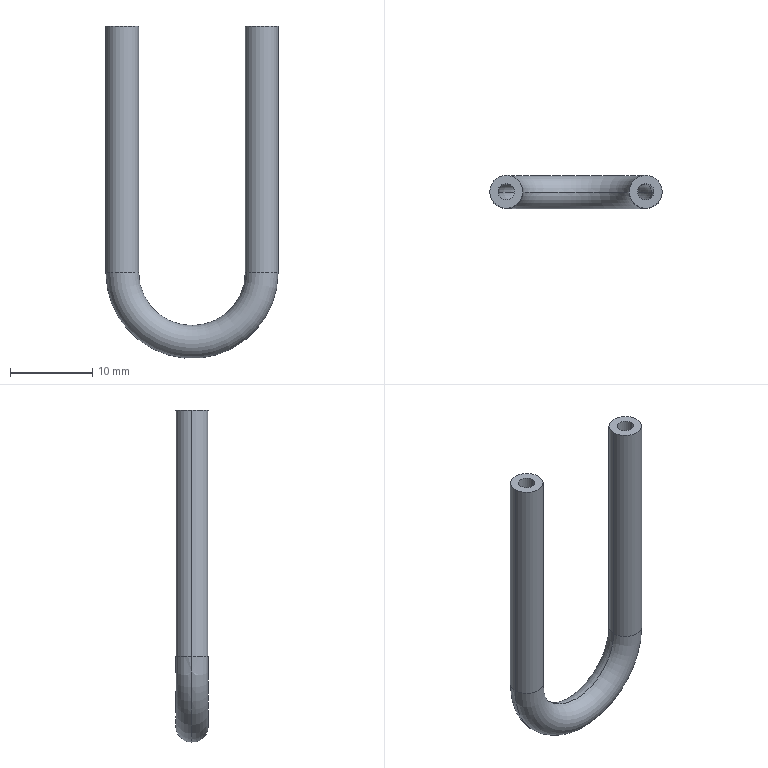Part | SolidWorks | features BaseBody 1 | 1 solid | 14 faces | box 21 x 4 x 40.5 mm | volume 817.162 mm3 | cylinder 8 | torus 4 | plane 2 | commonest cylinder face diameters 2 x4 4 x4
STEP:
#1=CARTESIAN_POINT('',(1.,0.,0.));
#2=VERTEX_POINT('',#1);
#3=CARTESIAN_POINT('',(-1.,0.,0.));
#4=VERTEX_POINT('',#3);
#5=CARTESIAN_POINT('',(0.,0.,0.));
#6=DIRECTION('',(0.,0.,1.));
#7=DIRECTION('',(1.,0.,0.));
#8=AXIS2_PLACEMENT_3D('',#5,#6,#7);
#9=CIRCLE('',#8,1.);
#10=EDGE_CURVE('',#2,#4,#9,.T.);
#11=ORIENTED_EDGE('',*,*,#10,.F.);
#12=CARTESIAN_POINT('',(0.,0.,0.));
#13=DIRECTION('',(0.,0.,1.));
#14=DIRECTION('',(-1.,0.,0.));
#15=AXIS2_PLACEMENT_3D('',#12,#13,#14);
#16=CIRCLE('',#15,1.);
#17=EDGE_CURVE('',#4,#2,#16,.T.);
#18=ORIENTED_EDGE('',*,*,#17,.F.);
#19=EDGE_LOOP('',(#11,#18));
#20=FACE_BOUND('',#19,.T.);
#21=CARTESIAN_POINT('',(2.,0.,0.));
#22=VERTEX_POINT('',#21);
#23=CARTESIAN_POINT('',(-2.,0.,0.));
#24=VERTEX_POINT('',#23);
#25=CARTESIAN_POINT('',(0.,0.,0.));
#26=DIRECTION('',(0.,0.,-1.));
#27=DIRECTION('',(1.,0.,0.));
#28=AXIS2_PLACEMENT_3D('',#25,#26,#27);
#29=CIRCLE('',#28,2.);
#30=EDGE_CURVE('',#22,#24,#29,.T.);
#31=ORIENTED_EDGE('',*,*,#30,.F.);
#32=CARTESIAN_POINT('',(0.,0.,0.));
#33=DIRECTION('',(0.,0.,-1.));
#34=DIRECTION('',(-1.,0.,0.));
#35=AXIS2_PLACEMENT_3D('',#32,#33,#34);
#36=CIRCLE('',#35,2.);
#37=EDGE_CURVE('',#24,#22,#36,.T.);
#38=ORIENTED_EDGE('',*,*,#37,.F.);
#39=EDGE_LOOP('',(#31,#38));
#40=FACE_OUTER_BOUND('',#39,.T.);
#41=CARTESIAN_POINT('',(0.,0.,0.));
#42=DIRECTION('',(0.,0.,1.));
#43=DIRECTION('',(1.,0.,0.));
#44=AXIS2_PLACEMENT_3D('',#41,#42,#43);
#45=PLANE('',#44);
#46=ADVANCED_FACE('',(#20,#40),#45,.T.);
#47=CARTESIAN_POINT('',(18.,0.,0.));
#48=VERTEX_POINT('',#47);
#49=CARTESIAN_POINT('',(16.,0.,0.));
#50=VERTEX_POINT('',#49);
#51=CARTESIAN_POINT('',(17.,0.,0.));
#52=DIRECTION('',(0.,0.,1.));
#53=DIRECTION('',(1.,0.,0.));
#54=AXIS2_PLACEMENT_3D('',#51,#52,#53);
#55=CIRCLE('',#54,1.);
#56=EDGE_CURVE('',#48,#50,#55,.T.);
#57=ORIENTED_EDGE('',*,*,#56,.F.);
#58=CARTESIAN_POINT('',(17.,0.,0.));
#59=DIRECTION('',(0.,0.,1.));
#60=DIRECTION('',(-1.,0.,0.));
#61=AXIS2_PLACEMENT_3D('',#58,#59,#60);
#62=CIRCLE('',#61,1.);
#63=EDGE_CURVE('',#50,#48,#62,.T.);
#64=ORIENTED_EDGE('',*,*,#63,.F.);
#65=EDGE_LOOP('',(#57,#64));
#66=FACE_BOUND('',#65,.T.);
#67=CARTESIAN_POINT('',(19.,0.,0.));
#68=VERTEX_POINT('',#67);
#69=CARTESIAN_POINT('',(15.,0.,0.));
#70=VERTEX_POINT('',#69);
#71=CARTESIAN_POINT('',(17.,0.,0.));
#72=DIRECTION('',(0.,0.,-1.));
#73=DIRECTION('',(1.,0.,0.));
#74=AXIS2_PLACEMENT_3D('',#71,#72,#73);
#75=CIRCLE('',#74,2.);
#76=EDGE_CURVE('',#68,#70,#75,.T.);
#77=ORIENTED_EDGE('',*,*,#76,.F.);
#78=CARTESIAN_POINT('',(17.,0.,0.));
#79=DIRECTION('',(0.,0.,-1.));
#80=DIRECTION('',(-1.,0.,0.));
#81=AXIS2_PLACEMENT_3D('',#78,#79,#80);
#82=CIRCLE('',#81,2.);
#83=EDGE_CURVE('',#70,#68,#82,.T.);
#84=ORIENTED_EDGE('',*,*,#83,.F.);
#85=EDGE_LOOP('',(#77,#84));
#86=FACE_OUTER_BOUND('',#85,.T.);
#87=CARTESIAN_POINT('',(17.,0.,0.));
#88=DIRECTION('',(0.,0.,1.));
#89=DIRECTION('',(1.,0.,0.));
#90=AXIS2_PLACEMENT_3D('',#87,#88,#89);
#91=PLANE('',#90);
#92=ADVANCED_FACE('',(#66,#86),#91,.T.);
#93=ORIENTED_EDGE('',*,*,#37,.T.);
#94=CARTESIAN_POINT('',(2.,0.,-30.));
#95=VERTEX_POINT('',#94);
#96=CARTESIAN_POINT('',(2.,0.,-30.));
#97=DIRECTION('',(0.,0.,1.));
#98=VECTOR('',#97,1000.);
#99=LINE('',#96,#98);
#100=EDGE_CURVE('',#95,#22,#99,.T.);
#101=ORIENTED_EDGE('',*,*,#100,.F.);
#102=CARTESIAN_POINT('',(-2.,0.,-30.));
#103=VERTEX_POINT('',#102);
#104=CARTESIAN_POINT('',(0.,0.,-30.));
#105=DIRECTION('',(0.,0.,-1.));
#106=DIRECTION('',(-1.,0.,0.));
#107=AXIS2_PLACEMENT_3D('',#104,#105,#106);
#108=CIRCLE('',#107,2.);
#109=EDGE_CURVE('',#103,#95,#108,.T.);
#110=ORIENTED_EDGE('',*,*,#109,.F.);
#111=CARTESIAN_POINT('',(-2.,0.,0.));
#112=DIRECTION('',(0.,0.,-1.));
#113=VECTOR('',#112,1000.);
#114=LINE('',#111,#113);
#115=EDGE_CURVE('',#24,#103,#114,.T.);
#116=ORIENTED_EDGE('',*,*,#115,.F.);
#117=EDGE_LOOP('',(#93,#101,#110,#116));
#118=FACE_OUTER_BOUND('',#117,.T.);
#119=CARTESIAN_POINT('',(0.,0.,-30.));
#120=DIRECTION('',(0.,0.,1.));
#121=DIRECTION('',(1.,0.,0.));
#122=AXIS2_PLACEMENT_3D('',#119,#120,#121);
#123=CYLINDRICAL_SURFACE('',#122,2.);
#124=ADVANCED_FACE('',(#118),#123,.T.);
#125=ORIENTED_EDGE('',*,*,#115,.T.);
#126=CARTESIAN_POINT('',(0.,0.,-30.));
#127=DIRECTION('',(0.,0.,-1.));
#128=DIRECTION('',(1.,0.,0.));
#129=AXIS2_PLACEMENT_3D('',#126,#127,#128);
#130=CIRCLE('',#129,2.);
#131=EDGE_CURVE('',#95,#103,#130,.T.);
#132=ORIENTED_EDGE('',*,*,#131,.F.);
#133=ORIENTED_EDGE('',*,*,#100,.T.);
#134=ORIENTED_EDGE('',*,*,#30,.T.);
#135=EDGE_LOOP('',(#125,#132,#133,#134));
#136=FACE_OUTER_BOUND('',#135,.T.);
#137=CARTESIAN_POINT('',(0.,0.,-30.));
#138=DIRECTION('',(0.,0.,1.));
#139=DIRECTION('',(1.,0.,0.));
#140=AXIS2_PLACEMENT_3D('',#137,#138,#139);
#141=CYLINDRICAL_SURFACE('',#140,2.);
#142=ADVANCED_FACE('',(#136),#141,.T.);
#143=CARTESIAN_POINT('',(1.,0.,-30.));
#144=VERTEX_POINT('',#143);
#145=CARTESIAN_POINT('',(-1.,0.,-30.));
#146=VERTEX_POINT('',#145);
#147=CARTESIAN_POINT('',(0.,0.,-30.));
#148=DIRECTION('',(0.,0.,1.));
#149=DIRECTION('',(1.,0.,0.));
#150=AXIS2_PLACEMENT_3D('',#147,#148,#149);
#151=CIRCLE('',#150,1.);
#152=EDGE_CURVE('',#144,#146,#151,.T.);
#153=ORIENTED_EDGE('',*,*,#152,.F.);
#154=CARTESIAN_POINT('',(1.,0.,0.));
#155=DIRECTION('',(0.,0.,-1.));
#156=VECTOR('',#155,1000.);
#157=LINE('',#154,#156);
#158=EDGE_CURVE('',#2,#144,#157,.T.);
#159=ORIENTED_EDGE('',*,*,#158,.F.);
#160=ORIENTED_EDGE('',*,*,#10,.T.);
#161=CARTESIAN_POINT('',(-1.,0.,-30.));
#162=DIRECTION('',(0.,0.,1.));
#163=VECTOR('',#162,1000.);
#164=LINE('',#161,#163);
#165=EDGE_CURVE('',#146,#4,#164,.T.);
#166=ORIENTED_EDGE('',*,*,#165,.F.);
#167=EDGE_LOOP('',(#153,#159,#160,#166));
#168=FACE_OUTER_BOUND('',#167,.T.);
#169=CARTESIAN_POINT('',(0.,0.,-30.));
#170=DIRECTION('',(0.,0.,1.));
#171=DIRECTION('',(1.,0.,0.));
#172=AXIS2_PLACEMENT_3D('',#169,#170,#171);
#173=CYLINDRICAL_SURFACE('',#172,1.);
#174=ADVANCED_FACE('',(#168),#173,.F.);
#175=CARTESIAN_POINT('',(0.,0.,-30.));
#176=DIRECTION('',(0.,0.,1.));
#177=DIRECTION('',(-1.,0.,0.));
#178=AXIS2_PLACEMENT_3D('',#175,#176,#177);
#179=CIRCLE('',#178,1.);
#180=EDGE_CURVE('',#146,#144,#179,.T.);
#181=ORIENTED_EDGE('',*,*,#180,.F.);
#182=ORIENTED_EDGE('',*,*,#165,.T.);
#183=ORIENTED_EDGE('',*,*,#17,.T.);
#184=ORIENTED_EDGE('',*,*,#158,.T.);
#185=EDGE_LOOP('',(#181,#182,#183,#184));
#186=FACE_OUTER_BOUND('',#185,.T.);
#187=CARTESIAN_POINT('',(0.,0.,-30.));
#188=DIRECTION('',(0.,0.,1.));
#189=DIRECTION('',(1.,0.,0.));
#190=AXIS2_PLACEMENT_3D('',#187,#188,#189);
#191=CYLINDRICAL_SURFACE('',#190,1.);
#192=ADVANCED_FACE('',(#186),#191,.F.);
#193=ORIENTED_EDGE('',*,*,#152,.T.);
#194=CARTESIAN_POINT('',(18.,0.000000068,-30.));
#195=VERTEX_POINT('',#194);
#196=CARTESIAN_POINT('',(8.5,0.,-30.));
#197=DIRECTION('',(0.,1.,0.));
#198=DIRECTION('',(1.,0.,0.000000003));
#199=AXIS2_PLACEMENT_3D('',#196,#197,#198);
#200=CIRCLE('',#199,9.5);
#201=EDGE_CURVE('',#195,#146,#200,.T.);
#202=ORIENTED_EDGE('',*,*,#201,.F.);
#203=CARTESIAN_POINT('',(16.,0.,-30.));
#204=VERTEX_POINT('',#203);
#205=CARTESIAN_POINT('',(17.,0.,-30.));
#206=DIRECTION('',(0.,0.,-1.));
#207=DIRECTION('',(-1.,0.,0.));
#208=AXIS2_PLACEMENT_3D('',#205,#206,#207);
#209=CIRCLE('',#208,1.);
#210=EDGE_CURVE('',#204,#195,#209,.T.);
#211=ORIENTED_EDGE('',*,*,#210,.F.);
#212=CARTESIAN_POINT('',(8.5,0.,-30.));
#213=DIRECTION('',(0.,-1.,0.));
#214=DIRECTION('',(-1.,0.,0.));
#215=AXIS2_PLACEMENT_3D('',#212,#213,#214);
#216=CIRCLE('',#215,7.5);
#217=EDGE_CURVE('',#144,#204,#216,.T.);
#218=ORIENTED_EDGE('',*,*,#217,.F.);
#219=EDGE_LOOP('',(#193,#202,#211,#218));
#220=FACE_OUTER_BOUND('',#219,.T.);
#221=CARTESIAN_POINT('',(8.5,0.,-30.));
#222=DIRECTION('',(0.,-1.,0.));
#223=DIRECTION('',(1.,0.,0.000000026));
#224=AXIS2_PLACEMENT_3D('',#221,#222,#223);
#225=TOROIDAL_SURFACE('',#224,8.5,1.);
#226=ADVANCED_FACE('',(#220),#225,.F.);
#227=ORIENTED_EDGE('',*,*,#180,.T.);
#228=ORIENTED_EDGE('',*,*,#217,.T.);
#229=CARTESIAN_POINT('',(17.,0.,-30.));
#230=DIRECTION('',(0.,0.,1.));
#231=DIRECTION('',(-1.,0.,0.));
#232=AXIS2_PLACEMENT_3D('',#229,#230,#231);
#233=CIRCLE('',#232,1.);
#234=EDGE_CURVE('',#204,#195,#233,.T.);
#235=ORIENTED_EDGE('',*,*,#234,.T.);
#236=ORIENTED_EDGE('',*,*,#201,.T.);
#237=EDGE_LOOP('',(#227,#228,#235,#236));
#238=FACE_OUTER_BOUND('',#237,.T.);
#239=CARTESIAN_POINT('',(8.5,0.,-30.));
#240=DIRECTION('',(0.,-1.,0.));
#241=DIRECTION('',(1.,0.,0.000000026));
#242=AXIS2_PLACEMENT_3D('',#239,#240,#241);
#243=TOROIDAL_SURFACE('',#242,8.5,1.);
#244=ADVANCED_FACE('',(#238),#243,.F.);
#245=CARTESIAN_POINT('',(19.,0.,-30.));
#246=VERTEX_POINT('',#245);
#247=CARTESIAN_POINT('',(15.,0.,-30.));
#248=VERTEX_POINT('',#247);
#249=CARTESIAN_POINT('',(17.,0.,-30.));
#250=DIRECTION('',(0.,0.,1.));
#251=DIRECTION('',(1.,0.,0.));
#252=AXIS2_PLACEMENT_3D('',#249,#250,#251);
#253=CIRCLE('',#252,2.);
#254=EDGE_CURVE('',#246,#248,#253,.T.);
#255=ORIENTED_EDGE('',*,*,#254,.F.);
#256=CARTESIAN_POINT('',(8.5,0.,-30.));
#257=DIRECTION('',(0.,-1.,0.));
#258=DIRECTION('',(-1.,0.,0.));
#259=AXIS2_PLACEMENT_3D('',#256,#257,#258);
#260=CIRCLE('',#259,10.5);
#261=EDGE_CURVE('',#103,#246,#260,.T.);
#262=ORIENTED_EDGE('',*,*,#261,.F.);
#263=ORIENTED_EDGE('',*,*,#109,.T.);
#264=CARTESIAN_POINT('',(8.5,0.,-30.));
#265=DIRECTION('',(0.,1.,0.));
#266=DIRECTION('',(1.,0.,0.));
#267=AXIS2_PLACEMENT_3D('',#264,#265,#266);
#268=CIRCLE('',#267,6.5);
#269=EDGE_CURVE('',#248,#95,#268,.T.);
#270=ORIENTED_EDGE('',*,*,#269,.F.);
#271=EDGE_LOOP('',(#255,#262,#263,#270));
#272=FACE_OUTER_BOUND('',#271,.T.);
#273=CARTESIAN_POINT('',(8.5,0.,-30.));
#274=DIRECTION('',(0.,1.,0.));
#275=DIRECTION('',(-1.,0.,0.));
#276=AXIS2_PLACEMENT_3D('',#273,#274,#275);
#277=TOROIDAL_SURFACE('',#276,8.5,2.);
#278=ADVANCED_FACE('',(#272),#277,.T.);
#279=ORIENTED_EDGE('',*,*,#269,.T.);
#280=ORIENTED_EDGE('',*,*,#131,.T.);
#281=ORIENTED_EDGE('',*,*,#261,.T.);
#282=CARTESIAN_POINT('',(17.,0.,-30.));
#283=DIRECTION('',(0.,0.,1.));
#284=DIRECTION('',(-1.,0.,0.));
#285=AXIS2_PLACEMENT_3D('',#282,#283,#284);
#286=CIRCLE('',#285,2.);
#287=EDGE_CURVE('',#248,#246,#286,.T.);
#288=ORIENTED_EDGE('',*,*,#287,.F.);
#289=EDGE_LOOP('',(#279,#280,#281,#288));
#290=FACE_OUTER_BOUND('',#289,.T.);
#291=CARTESIAN_POINT('',(8.5,0.,-30.));
#292=DIRECTION('',(0.,1.,0.));
#293=DIRECTION('',(-1.,0.,0.));
#294=AXIS2_PLACEMENT_3D('',#291,#292,#293);
#295=TOROIDAL_SURFACE('',#294,8.5,2.);
#296=ADVANCED_FACE('',(#290),#295,.T.);
#297=ORIENTED_EDGE('',*,*,#210,.T.);
#298=CARTESIAN_POINT('',(18.,0.,0.));
#299=DIRECTION('',(0.,0.,-1.));
#300=VECTOR('',#299,1000.);
#301=LINE('',#298,#300);
#302=EDGE_CURVE('',#48,#195,#301,.T.);
#303=ORIENTED_EDGE('',*,*,#302,.F.);
#304=ORIENTED_EDGE('',*,*,#56,.T.);
#305=CARTESIAN_POINT('',(16.,0.,-30.));
#306=DIRECTION('',(0.,0.,1.));
#307=VECTOR('',#306,1000.);
#308=LINE('',#305,#307);
#309=EDGE_CURVE('',#204,#50,#308,.T.);
#310=ORIENTED_EDGE('',*,*,#309,.F.);
#311=EDGE_LOOP('',(#297,#303,#304,#310));
#312=FACE_OUTER_BOUND('',#311,.T.);
#313=CARTESIAN_POINT('',(17.,0.,-30.));
#314=DIRECTION('',(0.,0.,1.));
#315=DIRECTION('',(1.,0.,0.));
#316=AXIS2_PLACEMENT_3D('',#313,#314,#315);
#317=CYLINDRICAL_SURFACE('',#316,1.);
#318=ADVANCED_FACE('',(#312),#317,.F.);
#319=ORIENTED_EDGE('',*,*,#309,.T.);
#320=ORIENTED_EDGE('',*,*,#63,.T.);
#321=ORIENTED_EDGE('',*,*,#302,.T.);
#322=ORIENTED_EDGE('',*,*,#234,.F.);
#323=EDGE_LOOP('',(#319,#320,#321,#322));
#324=FACE_OUTER_BOUND('',#323,.T.);
#325=CARTESIAN_POINT('',(17.,0.,-30.));
#326=DIRECTION('',(0.,0.,1.));
#327=DIRECTION('',(1.,0.,0.));
#328=AXIS2_PLACEMENT_3D('',#325,#326,#327);
#329=CYLINDRICAL_SURFACE('',#328,1.);
#330=ADVANCED_FACE('',(#324),#329,.F.);
#331=ORIENTED_EDGE('',*,*,#83,.T.);
#332=CARTESIAN_POINT('',(19.,0.,-30.));
#333=DIRECTION('',(0.,0.,1.));
#334=VECTOR('',#333,1000.);
#335=LINE('',#332,#334);
#336=EDGE_CURVE('',#246,#68,#335,.T.);
#337=ORIENTED_EDGE('',*,*,#336,.F.);
#338=ORIENTED_EDGE('',*,*,#254,.T.);
#339=CARTESIAN_POINT('',(15.,0.,0.));
#340=DIRECTION('',(0.,0.,-1.));
#341=VECTOR('',#340,1000.);
#342=LINE('',#339,#341);
#343=EDGE_CURVE('',#70,#248,#342,.T.);
#344=ORIENTED_EDGE('',*,*,#343,.F.);
#345=EDGE_LOOP('',(#331,#337,#338,#344));
#346=FACE_OUTER_BOUND('',#345,.T.);
#347=CARTESIAN_POINT('',(17.,0.,-30.));
#348=DIRECTION('',(0.,0.,1.));
#349=DIRECTION('',(1.,0.,0.));
#350=AXIS2_PLACEMENT_3D('',#347,#348,#349);
#351=CYLINDRICAL_SURFACE('',#350,2.);
#352=ADVANCED_FACE('',(#346),#351,.T.);
#353=ORIENTED_EDGE('',*,*,#343,.T.);
#354=ORIENTED_EDGE('',*,*,#287,.T.);
#355=ORIENTED_EDGE('',*,*,#336,.T.);
#356=ORIENTED_EDGE('',*,*,#76,.T.);
#357=EDGE_LOOP('',(#353,#354,#355,#356));
#358=FACE_OUTER_BOUND('',#357,.T.);
#359=CARTESIAN_POINT('',(17.,0.,-30.));
#360=DIRECTION('',(0.,0.,1.));
#361=DIRECTION('',(1.,0.,0.));
#362=AXIS2_PLACEMENT_3D('',#359,#360,#361);
#363=CYLINDRICAL_SURFACE('',#362,2.);
#364=ADVANCED_FACE('',(#358),#363,.T.);
#365=CLOSED_SHELL('',(#46,#92,#124,#142,#174,#192,#226,#244,#278,#296,#318,#330,#352,#364));
#366=MANIFOLD_SOLID_BREP('',#365);
#367=CARTESIAN_POINT('',(0.,0.,0.));
#368=DIRECTION('',(0.,0.,1.));
#369=DIRECTION('',(1.,0.,0.));
#370=AXIS2_PLACEMENT_3D('',#367,#368,#369);
#371=(LENGTH_UNIT()NAMED_UNIT(*)SI_UNIT(.MILLI.,.METRE.));
#372=UNCERTAINTY_MEASURE_WITH_UNIT(LENGTH_MEASURE(0.00001),#371,'','');
#373=(NAMED_UNIT(*)PLANE_ANGLE_UNIT()SI_UNIT($,.RADIAN.));
#374=(NAMED_UNIT(*)SI_UNIT($,.STERADIAN.)SOLID_ANGLE_UNIT());
#375=(GEOMETRIC_REPRESENTATION_CONTEXT(3)GLOBAL_UNCERTAINTY_ASSIGNED_CONTEXT((#372))GLOBAL_UNIT_ASSIGNED_CONTEXT((#371,#373,#374))REPRESENTATION_CONTEXT('',''));
#376=ADVANCED_BREP_SHAPE_REPRESENTATION('',(#366,#370),#375);